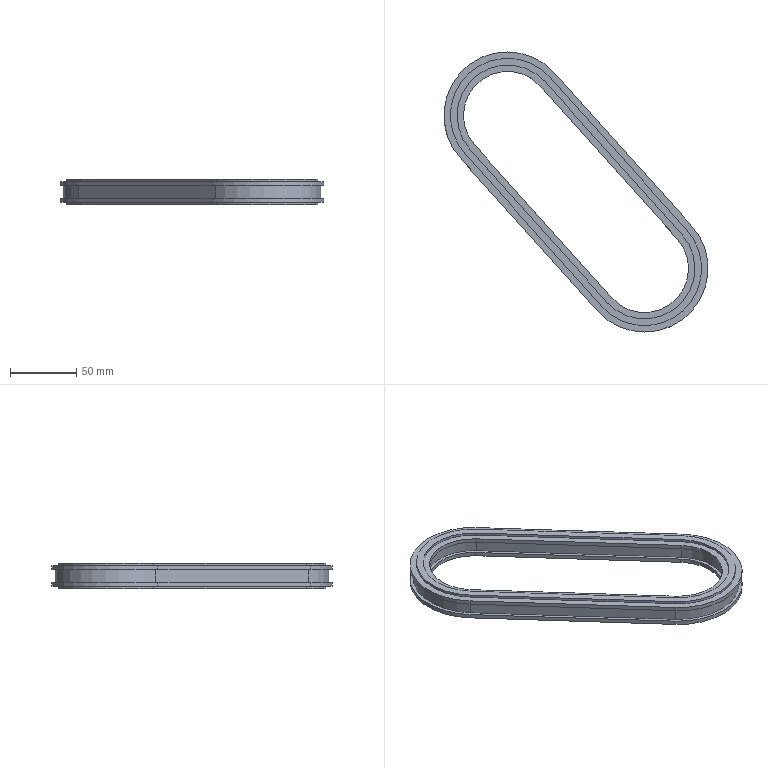Part | STEP file | Roller chain1 | 1 solid | 50 faces | box 199.55 x 211.673 x 19.6 mm | volume 116843 mm3 | plane 30 | cylinder 20 | commonest cylinder face diameters 66.643 x4 76.293 x4 86.453 x4 96.103 x4 71.213 x2 91.533 x2